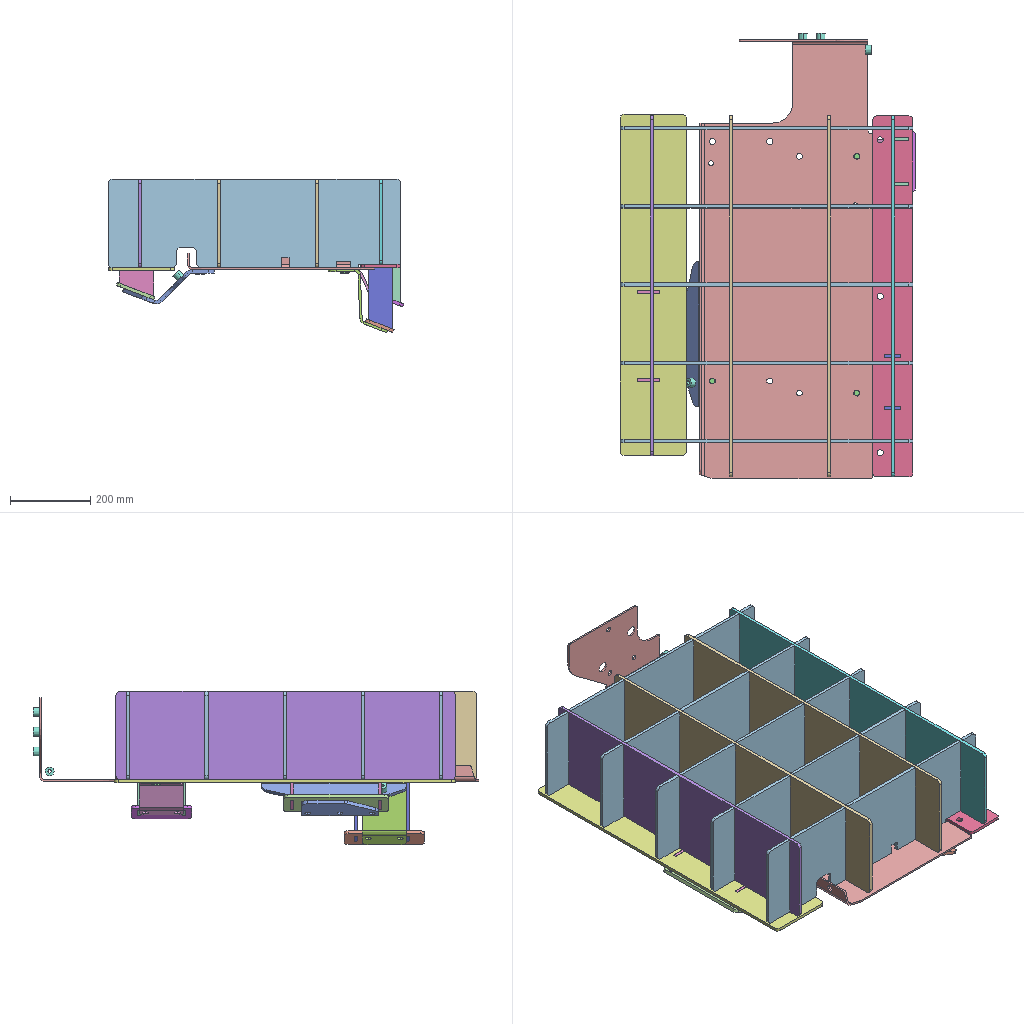Assembly | SolidWorks | 20 different items | 35 placed | box 737 x 1111 x 382 mm
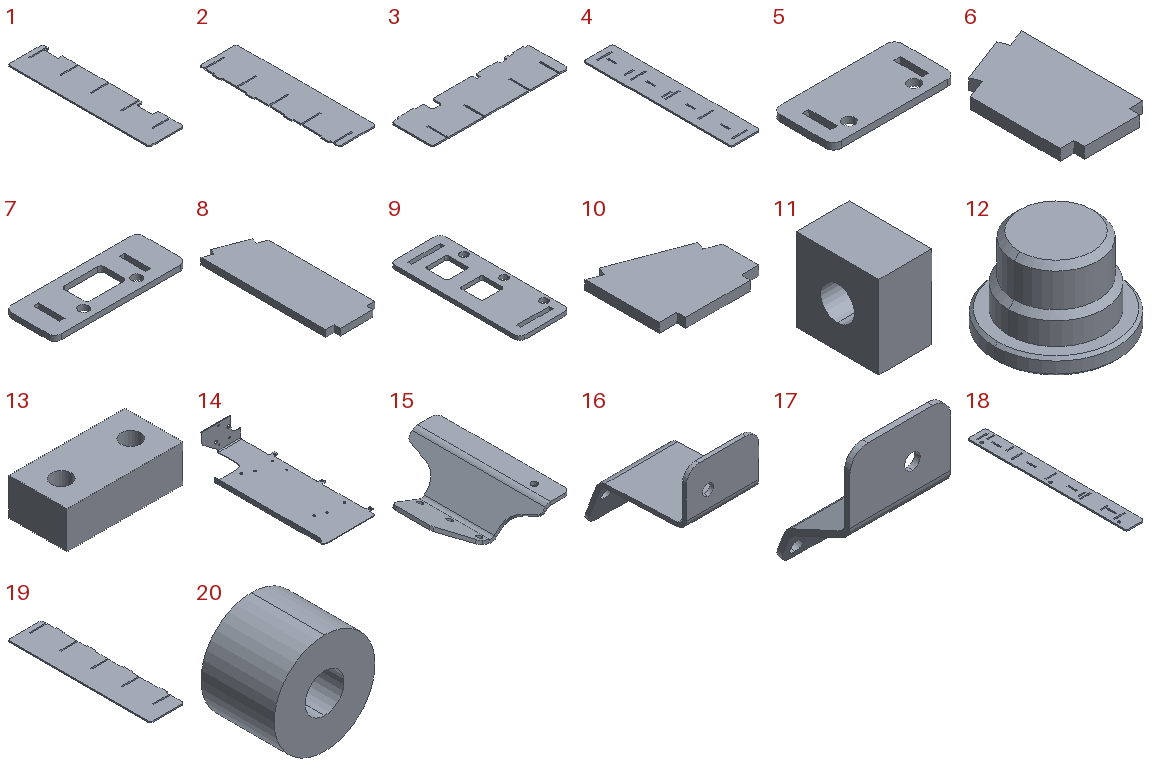Parts list (item | quantity | size | volume | features):
1 | x2 | 220 x 900 x 8 mm | 1500106 mm3 | features FlatPattern 1, SMBaseFlange 1, SheetMetal 1
2 | x1 | 227.5 x 847.5 x 8 mm | 1466273 mm3 | features FlatPattern 1, SMBaseFlange 1, SheetMetal 1
3 | x5 | 730 x 227.5 x 8 mm | 1230929 mm3 | features FlatPattern 1, SMBaseFlange 1, SheetMetal 1
4 | x1 | 165 x 850 x 8 mm | 1074273 mm3 | features FlatPattern 1, SMBaseFlange 1, SheetMetal 1
5 | x1 | 150 x 75 x 8 mm | 82006 mm3 | features FlatPattern 1, SMBaseFlange 1, SheetMetal 1
6 | x2 | 60 x 97.324 x 8 mm | 41194 mm3 | features FlatPattern 1, SMBaseFlange 1, SheetMetal 1
7 | x1 | 200 x 75 x 8 mm | 92818 mm3 | features FlatPattern 1, SMBaseFlange 1, SheetMetal 1
8 | x2 | 60 x 162.47 x 8 mm | 72422 mm3 | features FlatPattern 1, SMBaseFlange 1, SheetMetal 1
9 | x1 | 100 x 260 x 8 mm | 162695 mm3 | features FlatPattern 1, SMBaseFlange 1, SheetMetal 1
10 | x2 | 85 x 73.23 x 8 mm | 39231 mm3 | features FlatPattern 1, SMBaseFlange 1, SheetMetal 1
11 | x2 | 16 x 25 x 25 mm | 8693 mm3 | features FlatPattern 1, HoleWzd 1, SMBaseFlange 1, SheetMetal 1
12 | x3 | 22 x 22 x 15 mm | 3447 mm3 | features Chamfer 2, Revolution 1
13 | x1 | 50 x 25 x 16 mm | 18184 mm3 | features FlatPattern 1, HoleWzd 1, SMBaseFlange 1, SheetMetal 1
14 | x1 | 466 x 1095 x 209 mm | 2221279 mm3 | features ICE 3, EdgeFlange 2, Fillet 2, FlatPattern 1, Fold 1, SMBaseFlange 1, SheetMetal 1, UnFold 1
15 | x1 | 228.191 x 360 x 86.08 mm | 576427 mm3 | features SM3dBend 2, FlatPattern 1, SMBaseFlange 1, SheetMetal 1
16 | x1 | 110 x 157.607 x 148 mm | 171596 mm3 | features Fillet 2, ICE 2, FlatPattern 1, SMBaseFlange 1, SheetMetal 1
17 | x1 | 110 x 83.637 x 145 mm | 117261 mm3 | features Fillet 2, ICE 2, FlatPattern 1, SMBaseFlange 1, SheetMetal 1
18 | x1 | 100 x 900 x 8 mm | 672832 mm3 | features FlatPattern 1, SMBaseFlange 1, SheetMetal 1
19 | x1 | 219.5 x 900 x 8 mm | 1503633 mm3 | features FlatPattern 1, SMBaseFlange 1, SheetMetal 1
20 | x5 | 22 x 16 x 22 mm | 5174 mm3 | features Extrusion 1, HoleWzd 1
Mates (type | each side: item.copy, entity, surface, feature):
Coincident | 14.1 face plane Base-Flange1 | 15.1 face plane Base-Flange1
Concentric | 14.1 face cylinder Base-Flange1 | 15.1 face cylinder Base-Flange1
Parallel | 14.1 face plane Edge-Flange1 | 15.1 face plane Base-Flange1
Coincident | 14.1 face plane Base-Flange1 | 16.1 face plane Base-Flange1
Concentric | 14.1 face cylinder Base-Flange1 | 16.1 face cylinder Cut-Extrude1
Parallel | 14.1 face plane Base-Flange1 | 16.1 face plane Base-Flange1
Coincident | 14.1 face plane Base-Flange1 | 17.1 face plane Base-Flange1
Concentric | 14.1 face cylinder Base-Flange1 | 17.1 face cylinder Cut-Extrude1
Parallel | 14.1 face plane Base-Flange1 | 17.1 face plane Base-Flange1
Coincident | 14.1 face plane Edge-Flange2 | 20.1 face plane Boss-Extrude1
DistanceDim | 20.1 face cylinder Boss-Extrude1 | 14.1 face plane Base-Flange1
DistanceDim | 20.1 face cylinder Boss-Extrude1 | 14.1 face plane Cut-Extrude2
Coincident | 14.1 face plane Edge-Flange2 | 20.2 face plane Boss-Extrude1
DistanceDim | 20.2 face cylinder Boss-Extrude1 | 14.1 face plane Cut-Extrude2
DistanceDim | 20.1 face cylinder Boss-Extrude1 | 20.2 face cylinder Boss-Extrude1
Coincident | 14.1 face plane Edge-Flange2 | 20.3 face plane Boss-Extrude1
DistanceDim | 20.3 face cylinder Boss-Extrude1 | 14.1 face plane Cut-Extrude2
DistanceDim | 20.3 face cylinder Boss-Extrude1 | 14.1 face plane Base-Flange1
DistanceDim | 14.1 face plane Edge-Flange2 | 20.4 face cylinder Boss-Extrude1
DistanceDim | 14.1 face plane Base-Flange1 | 20.4 face cylinder Boss-Extrude1
Coincident | 15.1 face plane Base-Flange1 | 20.5 face plane Boss-Extrude1
DistanceDim | 15.1 face plane Base-Flange1 | 20.5 face cylinder Boss-Extrude1
DistanceDim | 20.5 face cylinder Boss-Extrude1 | 15.1 edge
Coincident | 15.1 face plane Base-Flange1 | 11.1 face plane Base-Flange1
DistanceDim | 11.1 face cylinder M12 Tapped Hole1 | 15.1 face plane Base-Flange1 | 2 times
Coincident | 15.1 face plane Base-Flange1 | 11.2 face plane Base-Flange1
Coincident | 11.1 face plane Base-Flange1 | 11.2 face plane Base-Flange1
DistanceDim | 11.1 face cylinder M12 Tapped Hole1 | 11.2 face cylinder M12 Tapped Hole1
Parallel | 15.1 face plane Base-Flange1 | 11.1 face plane Base-Flange1
Coincident | 16.1 face plane Base-Flange1 | 13.1 face plane Base-Flange1
DistanceDim | 13.1 face cylinder M10 Tapped Hole1 | 16.1 face plane Base-Flange1
DistanceDim | 13.1 face plane Base-Flange1 | 16.1 face plane Base-Flange1
Parallel | 16.1 face plane Base-Flange1 | 13.1 face plane Base-Flange1
Coincident | 15.1 face plane Base-Flange1 | 12.1 face plane Revolve1
Concentric | 15.1 face cylinder Base-Flange1 | 12.1 face cylinder Revolve1
Concentric | 16.1 face cylinder Cut-Extrude1 | 12.2 face cylinder Revolve1
Coincident | 16.1 face plane Base-Flange1 | 12.2 face plane Revolve1
Concentric | 17.1 face cylinder Cut-Extrude1 | 12.3 face cylinder Revolve1
Coincident | 17.1 face plane Base-Flange1 | 12.3 face plane Revolve1
InPlace | 14.1 face plane Base-Flange1 | 18.1 plane
InPlace | 3.1 plane | assembly plane
InPlace | 3.2 face plane Base-Flange1 | 4.1 plane
InPlace | 17.1 face plane Base-Flange1 | 5.1 plane
InPlace | 6.1 plane | assembly plane
InPlace | 16.1 face plane Base-Flange1 | 7.1 plane
InPlace | 16.1 face plane Base-Flange1 | 8.1 plane
InPlace | 15.1 face plane Base-Flange1 | 9.1 plane
InPlace | 15.1 face plane Base-Flange1 | 10.1 plane
InPlace | 19.1 plane | assembly plane
InPlace | 1.1 plane | assembly plane
InPlace | 2.1 plane | assembly plane